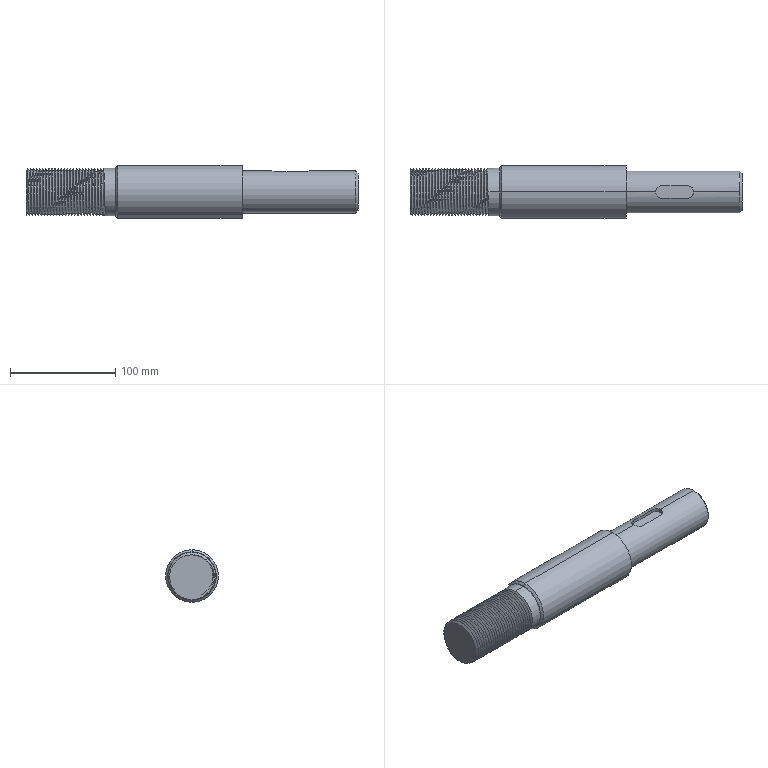Part | SolidWorks | 1 solid | 25 faces | box 315.002 x 50 x 50 mm | volume 494133 mm3 | cylinder 10 | plane 9 | cone 4 | spline 2 | commonest cylinder face diameters 12 x3 45 x3 40 x2 50 x2